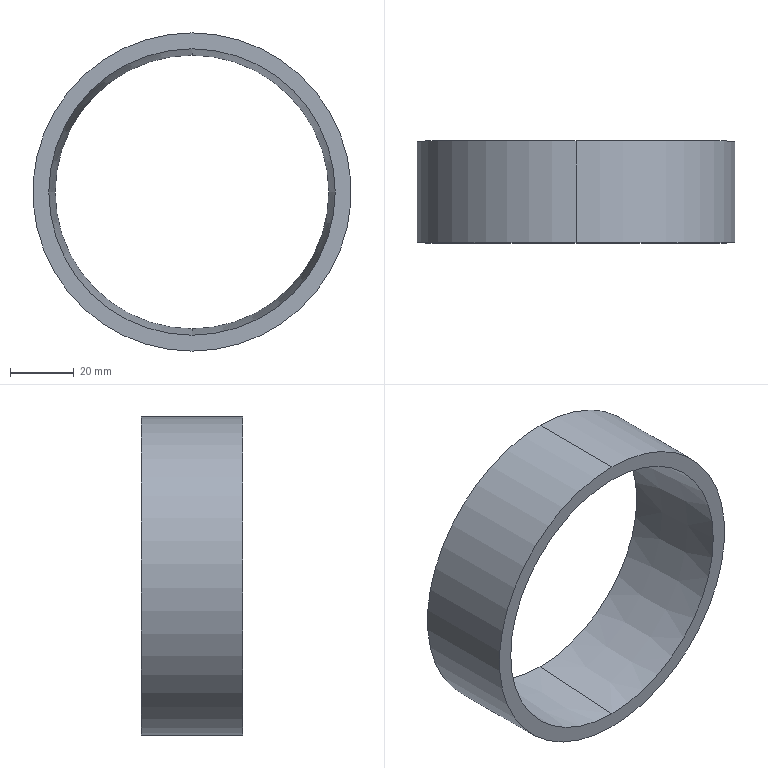Part | SolidWorks | features Revolution 1 | 1 solid | 6 faces | box 100 x 32 x 100 mm | volume 56666 mm3 | cone 2 | cylinder 2 | plane 2 | commonest cylinder face diameters 100 x2
STEP:
#1=CARTESIAN_POINT('',(0.,32.,43.));
#2=VERTEX_POINT('',#1);
#3=CARTESIAN_POINT('',(0.,32.,-43.));
#4=VERTEX_POINT('',#3);
#5=CARTESIAN_POINT('',(0.,32.,0.));
#6=DIRECTION('',(0.,-1.,0.));
#7=DIRECTION('',(0.,0.,-1.));
#8=AXIS2_PLACEMENT_3D('',#5,#6,#7);
#9=CIRCLE('',#8,43.);
#10=EDGE_CURVE('',#2,#4,#9,.T.);
#11=ORIENTED_EDGE('',*,*,#10,.F.);
#12=CARTESIAN_POINT('',(0.,0.,45.));
#13=VERTEX_POINT('',#12);
#14=CARTESIAN_POINT('',(0.,32.,43.));
#15=DIRECTION('',(0.,-0.9981,0.06238));
#16=VECTOR('',#15,1000.);
#17=LINE('',#14,#16);
#18=EDGE_CURVE('',#2,#13,#17,.T.);
#19=ORIENTED_EDGE('',*,*,#18,.T.);
#20=CARTESIAN_POINT('',(0.,0.,-45.));
#21=VERTEX_POINT('',#20);
#22=CARTESIAN_POINT('',(0.,0.,0.));
#23=DIRECTION('',(0.,-1.,0.));
#24=DIRECTION('',(0.,0.,-1.));
#25=AXIS2_PLACEMENT_3D('',#22,#23,#24);
#26=CIRCLE('',#25,45.);
#27=EDGE_CURVE('',#13,#21,#26,.T.);
#28=ORIENTED_EDGE('',*,*,#27,.T.);
#29=CARTESIAN_POINT('',(0.,32.,-43.));
#30=DIRECTION('',(0.,-0.9981,-0.06238));
#31=VECTOR('',#30,1000.);
#32=LINE('',#29,#31);
#33=EDGE_CURVE('',#4,#21,#32,.T.);
#34=ORIENTED_EDGE('',*,*,#33,.F.);
#35=EDGE_LOOP('',(#11,#19,#28,#34));
#36=FACE_OUTER_BOUND('',#35,.T.);
#37=CARTESIAN_POINT('',(0.,32.,0.));
#38=DIRECTION('',(0.,-1.,0.));
#39=DIRECTION('',(0.,0.,-1.));
#40=AXIS2_PLACEMENT_3D('',#37,#38,#39);
#41=CONICAL_SURFACE('',#40,43.,0.06242);
#42=ADVANCED_FACE('',(#36),#41,.F.);
#43=CARTESIAN_POINT('',(0.,32.,-50.));
#44=VERTEX_POINT('',#43);
#45=CARTESIAN_POINT('',(0.,32.,50.));
#46=VERTEX_POINT('',#45);
#47=CARTESIAN_POINT('',(0.,32.,0.));
#48=DIRECTION('',(0.,-1.,0.));
#49=DIRECTION('',(0.,0.,-1.));
#50=AXIS2_PLACEMENT_3D('',#47,#48,#49);
#51=CIRCLE('',#50,50.);
#52=EDGE_CURVE('',#44,#46,#51,.T.);
#53=ORIENTED_EDGE('',*,*,#52,.T.);
#54=CARTESIAN_POINT('',(0.,0.,50.));
#55=VERTEX_POINT('',#54);
#56=CARTESIAN_POINT('',(0.,0.,50.));
#57=DIRECTION('',(0.,-1.,0.));
#58=VECTOR('',#57,1000.);
#59=LINE('',#56,#58);
#60=EDGE_CURVE('',#46,#55,#59,.T.);
#61=ORIENTED_EDGE('',*,*,#60,.T.);
#62=CARTESIAN_POINT('',(0.,0.,-50.));
#63=VERTEX_POINT('',#62);
#64=CARTESIAN_POINT('',(0.,0.,0.));
#65=DIRECTION('',(0.,-1.,0.));
#66=DIRECTION('',(0.,0.,-1.));
#67=AXIS2_PLACEMENT_3D('',#64,#65,#66);
#68=CIRCLE('',#67,50.);
#69=EDGE_CURVE('',#63,#55,#68,.T.);
#70=ORIENTED_EDGE('',*,*,#69,.F.);
#71=CARTESIAN_POINT('',(0.,0.,-50.));
#72=DIRECTION('',(0.,-1.,0.));
#73=VECTOR('',#72,1000.);
#74=LINE('',#71,#73);
#75=EDGE_CURVE('',#44,#63,#74,.T.);
#76=ORIENTED_EDGE('',*,*,#75,.F.);
#77=EDGE_LOOP('',(#53,#61,#70,#76));
#78=FACE_OUTER_BOUND('',#77,.T.);
#79=CARTESIAN_POINT('',(0.,0.,0.));
#80=DIRECTION('',(0.,-1.,0.));
#81=DIRECTION('',(0.,0.,-1.));
#82=AXIS2_PLACEMENT_3D('',#79,#80,#81);
#83=CYLINDRICAL_SURFACE('',#82,50.);
#84=ADVANCED_FACE('',(#78),#83,.T.);
#85=ORIENTED_EDGE('',*,*,#60,.F.);
#86=CARTESIAN_POINT('',(0.,32.,0.));
#87=DIRECTION('',(0.,-1.,0.));
#88=DIRECTION('',(0.,0.,-1.));
#89=AXIS2_PLACEMENT_3D('',#86,#87,#88);
#90=CIRCLE('',#89,50.);
#91=EDGE_CURVE('',#46,#44,#90,.T.);
#92=ORIENTED_EDGE('',*,*,#91,.T.);
#93=ORIENTED_EDGE('',*,*,#75,.T.);
#94=CARTESIAN_POINT('',(0.,0.,0.));
#95=DIRECTION('',(0.,-1.,0.));
#96=DIRECTION('',(0.,0.,-1.));
#97=AXIS2_PLACEMENT_3D('',#94,#95,#96);
#98=CIRCLE('',#97,50.);
#99=EDGE_CURVE('',#55,#63,#98,.T.);
#100=ORIENTED_EDGE('',*,*,#99,.F.);
#101=EDGE_LOOP('',(#85,#92,#93,#100));
#102=FACE_OUTER_BOUND('',#101,.T.);
#103=CARTESIAN_POINT('',(0.,0.,0.));
#104=DIRECTION('',(0.,-1.,0.));
#105=DIRECTION('',(0.,0.,-1.));
#106=AXIS2_PLACEMENT_3D('',#103,#104,#105);
#107=CYLINDRICAL_SURFACE('',#106,50.);
#108=ADVANCED_FACE('',(#102),#107,.T.);
#109=ORIENTED_EDGE('',*,*,#69,.T.);
#110=ORIENTED_EDGE('',*,*,#99,.T.);
#111=EDGE_LOOP('',(#109,#110));
#112=FACE_OUTER_BOUND('',#111,.T.);
#113=CARTESIAN_POINT('',(0.,0.,0.));
#114=DIRECTION('',(0.,-1.,0.));
#115=DIRECTION('',(0.,0.,-1.));
#116=AXIS2_PLACEMENT_3D('',#113,#114,#115);
#117=CIRCLE('',#116,45.);
#118=EDGE_CURVE('',#21,#13,#117,.T.);
#119=ORIENTED_EDGE('',*,*,#118,.F.);
#120=ORIENTED_EDGE('',*,*,#27,.F.);
#121=EDGE_LOOP('',(#119,#120));
#122=FACE_BOUND('',#121,.T.);
#123=CARTESIAN_POINT('',(45.,0.,0.));
#124=DIRECTION('',(0.,-1.,0.));
#125=DIRECTION('',(0.,0.,-1.));
#126=AXIS2_PLACEMENT_3D('',#123,#124,#125);
#127=PLANE('',#126);
#128=ADVANCED_FACE('',(#112,#122),#127,.T.);
#129=ORIENTED_EDGE('',*,*,#18,.F.);
#130=CARTESIAN_POINT('',(0.,32.,0.));
#131=DIRECTION('',(0.,-1.,0.));
#132=DIRECTION('',(0.,0.,-1.));
#133=AXIS2_PLACEMENT_3D('',#130,#131,#132);
#134=CIRCLE('',#133,43.);
#135=EDGE_CURVE('',#4,#2,#134,.T.);
#136=ORIENTED_EDGE('',*,*,#135,.F.);
#137=ORIENTED_EDGE('',*,*,#33,.T.);
#138=ORIENTED_EDGE('',*,*,#118,.T.);
#139=EDGE_LOOP('',(#129,#136,#137,#138));
#140=FACE_OUTER_BOUND('',#139,.T.);
#141=CARTESIAN_POINT('',(0.,32.,0.));
#142=DIRECTION('',(0.,-1.,0.));
#143=DIRECTION('',(0.,0.,-1.));
#144=AXIS2_PLACEMENT_3D('',#141,#142,#143);
#145=CONICAL_SURFACE('',#144,43.,0.06242);
#146=ADVANCED_FACE('',(#140),#145,.F.);
#147=ORIENTED_EDGE('',*,*,#135,.T.);
#148=ORIENTED_EDGE('',*,*,#10,.T.);
#149=EDGE_LOOP('',(#147,#148));
#150=FACE_BOUND('',#149,.T.);
#151=ORIENTED_EDGE('',*,*,#52,.F.);
#152=ORIENTED_EDGE('',*,*,#91,.F.);
#153=EDGE_LOOP('',(#151,#152));
#154=FACE_OUTER_BOUND('',#153,.T.);
#155=CARTESIAN_POINT('',(43.,32.,0.));
#156=DIRECTION('',(0.,1.,0.));
#157=DIRECTION('',(0.,0.,1.));
#158=AXIS2_PLACEMENT_3D('',#155,#156,#157);
#159=PLANE('',#158);
#160=ADVANCED_FACE('',(#150,#154),#159,.T.);
#161=CLOSED_SHELL('',(#42,#84,#108,#128,#146,#160));
#162=MANIFOLD_SOLID_BREP('',#161);
#163=CARTESIAN_POINT('',(0.,0.,0.));
#164=DIRECTION('',(0.,0.,1.));
#165=DIRECTION('',(1.,0.,0.));
#166=AXIS2_PLACEMENT_3D('',#163,#164,#165);
#167=(LENGTH_UNIT()NAMED_UNIT(*)SI_UNIT(.MILLI.,.METRE.));
#168=UNCERTAINTY_MEASURE_WITH_UNIT(LENGTH_MEASURE(0.00001),#167,'','');
#169=(NAMED_UNIT(*)PLANE_ANGLE_UNIT()SI_UNIT($,.RADIAN.));
#170=(NAMED_UNIT(*)SI_UNIT($,.STERADIAN.)SOLID_ANGLE_UNIT());
#171=(GEOMETRIC_REPRESENTATION_CONTEXT(3)GLOBAL_UNCERTAINTY_ASSIGNED_CONTEXT((#168))GLOBAL_UNIT_ASSIGNED_CONTEXT((#167,#169,#170))REPRESENTATION_CONTEXT('',''));
#172=ADVANCED_BREP_SHAPE_REPRESENTATION('',(#162,#166),#171);